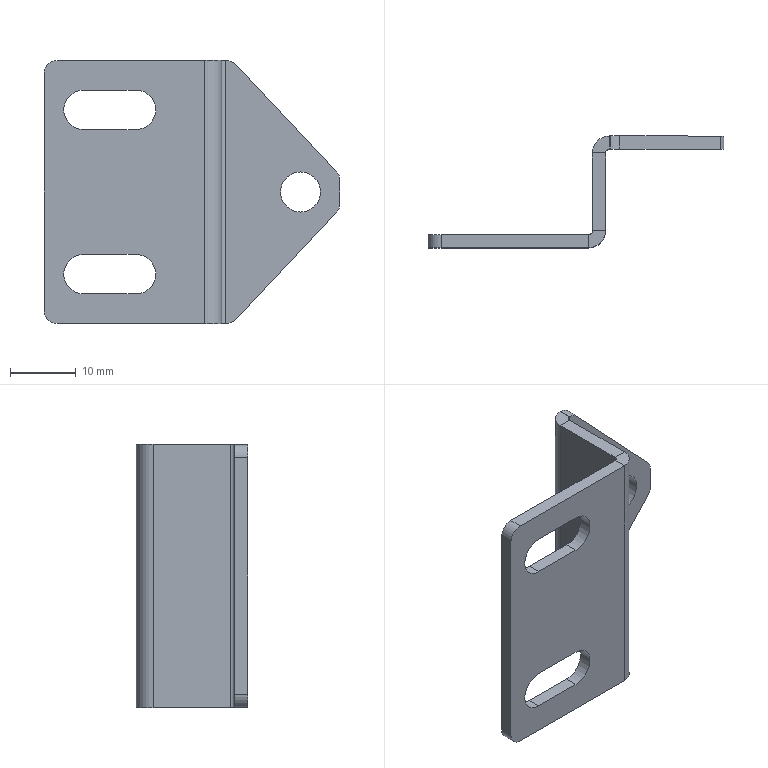Part | STEP file | 1 solid | 40 faces | box 45 x 17 x 40 mm | volume 3748 mm3 | plane 24 | cylinder 16 | commonest cylinder face diameters 4 x6 6 x4 1.2 x2 5.2 x2 6.1 x2